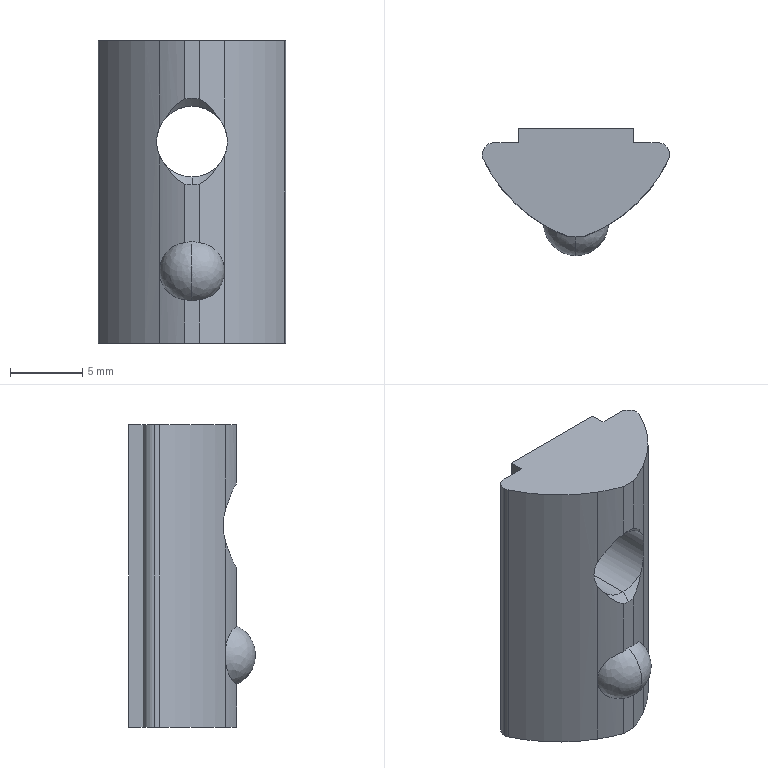Part | SolidWorks | features BaseBody 1 | 1 solid | 30 faces | box 13.001 x 8.797 x 21 mm | volume 1304 mm3 | cylinder 13 | plane 10 | cone 5 | spline 2 | commonest cylinder face diameters 20.854 x8 1.6 x3 4.917 x2
STEP:
#1=CARTESIAN_POINT('',(-0.0005,-8.797,-16.));
#2=VERTEX_POINT('',#1);
#3=CARTESIAN_POINT('',(-0.0005,-7.5,-18.038));
#4=VERTEX_POINT('',#3);
#5=CARTESIAN_POINT('',(-0.0005,-6.547,-16.));
#6=DIRECTION('',(1.,0.,0.));
#7=DIRECTION('',(0.,-1.,0.));
#8=AXIS2_PLACEMENT_3D('',#5,#6,#7);
#9=CIRCLE('',#8,2.25);
#10=EDGE_CURVE('',#2,#4,#9,.T.);
#11=ORIENTED_EDGE('',*,*,#10,.F.);
#12=CARTESIAN_POINT('',(-0.0005,-7.5,-13.962));
#13=VERTEX_POINT('',#12);
#14=CARTESIAN_POINT('',(-0.0005,-6.547,-16.));
#15=DIRECTION('',(-1.,0.,0.));
#16=DIRECTION('',(0.,-1.,0.));
#17=AXIS2_PLACEMENT_3D('',#14,#15,#16);
#18=CIRCLE('',#17,2.25);
#19=EDGE_CURVE('',#2,#13,#18,.T.);
#20=ORIENTED_EDGE('',*,*,#19,.T.);
#21=CARTESIAN_POINT('',(-0.5,-7.5,-14.024));
#22=VERTEX_POINT('',#21);
#23=CARTESIAN_POINT('',(-0.0005,-7.5,-16.));
#24=DIRECTION('',(0.,-1.,0.));
#25=DIRECTION('',(0.,0.,-1.));
#26=AXIS2_PLACEMENT_3D('',#23,#24,#25);
#27=CIRCLE('',#26,2.038);
#28=EDGE_CURVE('',#13,#22,#27,.T.);
#29=ORIENTED_EDGE('',*,*,#28,.T.);
#30=CARTESIAN_POINT('',(-2.246,-6.689,-16.));
#31=VERTEX_POINT('',#30);
#32=CARTESIAN_POINT('',(-0.5,-7.5,-14.024));
#33=CARTESIAN_POINT('',(-0.7396,-7.415,-14.043));
#34=CARTESIAN_POINT('',(-0.9674,-7.323,-14.106));
#35=CARTESIAN_POINT('',(-1.286,-7.184,-14.262));
#36=CARTESIAN_POINT('',(-1.386,-7.138,-14.324));
#37=CARTESIAN_POINT('',(-1.573,-7.049,-14.466));
#38=CARTESIAN_POINT('',(-1.662,-7.005,-14.548));
#39=CARTESIAN_POINT('',(-1.821,-6.924,-14.727));
#40=CARTESIAN_POINT('',(-1.892,-6.886,-14.824));
#41=CARTESIAN_POINT('',(-2.017,-6.819,-15.032));
#42=CARTESIAN_POINT('',(-2.071,-6.789,-15.144));
#43=CARTESIAN_POINT('',(-2.158,-6.74,-15.377));
#44=CARTESIAN_POINT('',(-2.19,-6.721,-15.497));
#45=CARTESIAN_POINT('',(-2.235,-6.696,-15.744));
#46=CARTESIAN_POINT('',(-2.246,-6.689,-15.872));
#47=CARTESIAN_POINT('',(-2.246,-6.689,-16.));
#48=B_SPLINE_CURVE_WITH_KNOTS('',3,(#32,#33,#34,#35,#36,#37,#38,#39,#40,#41,#42,#43,#44,#45,#46,#47),.UNSPECIFIED.,.F.,.F.,(4,2,2,2,2,2,2,4),(0.,0.0007548,0.001132,0.00151,0.001887,0.002264,0.002642,0.003019),.UNSPECIFIED.);
#49=EDGE_CURVE('',#22,#31,#48,.T.);
#50=ORIENTED_EDGE('',*,*,#49,.T.);
#51=CARTESIAN_POINT('',(-0.5,-7.5,-17.976));
#52=VERTEX_POINT('',#51);
#53=CARTESIAN_POINT('',(-0.5,-7.5,-17.976));
#54=CARTESIAN_POINT('',(-0.7396,-7.415,-17.957));
#55=CARTESIAN_POINT('',(-0.9674,-7.323,-17.894));
#56=CARTESIAN_POINT('',(-1.286,-7.184,-17.738));
#57=CARTESIAN_POINT('',(-1.386,-7.138,-17.676));
#58=CARTESIAN_POINT('',(-1.573,-7.049,-17.534));
#59=CARTESIAN_POINT('',(-1.662,-7.005,-17.452));
#60=CARTESIAN_POINT('',(-1.821,-6.924,-17.273));
#61=CARTESIAN_POINT('',(-1.892,-6.886,-17.176));
#62=CARTESIAN_POINT('',(-2.017,-6.819,-16.968));
#63=CARTESIAN_POINT('',(-2.071,-6.789,-16.856));
#64=CARTESIAN_POINT('',(-2.158,-6.74,-16.623));
#65=CARTESIAN_POINT('',(-2.19,-6.721,-16.503));
#66=CARTESIAN_POINT('',(-2.235,-6.696,-16.256));
#67=CARTESIAN_POINT('',(-2.246,-6.689,-16.128));
#68=CARTESIAN_POINT('',(-2.246,-6.689,-16.));
#69=B_SPLINE_CURVE_WITH_KNOTS('',3,(#53,#54,#55,#56,#57,#58,#59,#60,#61,#62,#63,#64,#65,#66,#67,#68),.UNSPECIFIED.,.F.,.F.,(4,2,2,2,2,2,2,4),(0.,0.0007548,0.001132,0.00151,0.001887,0.002264,0.002642,0.003019),.UNSPECIFIED.);
#70=EDGE_CURVE('',#52,#31,#69,.T.);
#71=ORIENTED_EDGE('',*,*,#70,.F.);
#72=CARTESIAN_POINT('',(-0.0005,-7.5,-16.));
#73=DIRECTION('',(0.,1.,0.));
#74=DIRECTION('',(0.,0.,-1.));
#75=AXIS2_PLACEMENT_3D('',#72,#73,#74);
#76=CIRCLE('',#75,2.038);
#77=EDGE_CURVE('',#4,#52,#76,.T.);
#78=ORIENTED_EDGE('',*,*,#77,.F.);
#79=EDGE_LOOP('',(#11,#20,#29,#50,#71,#78));
#80=FACE_OUTER_BOUND('',#79,.T.);
#81=CARTESIAN_POINT('',(-0.0005,-8.797,-16.));
#82=CARTESIAN_POINT('',(-0.0005,-8.797,-16.));
#83=CARTESIAN_POINT('',(-0.0005,-8.797,-16.));
#84=CARTESIAN_POINT('',(-0.0005,-8.797,-16.));
#85=CARTESIAN_POINT('',(-0.0005,-8.797,-14.738));
#86=CARTESIAN_POINT('',(-2.525,-8.797,-14.738));
#87=CARTESIAN_POINT('',(-2.525,-8.797,-17.262));
#88=CARTESIAN_POINT('',(-0.0005,-8.797,-17.262));
#89=CARTESIAN_POINT('',(-0.0005,-7.929,-13.822));
#90=CARTESIAN_POINT('',(-4.357,-7.929,-13.822));
#91=CARTESIAN_POINT('',(-4.357,-7.929,-18.178));
#92=CARTESIAN_POINT('',(-0.0005,-7.929,-18.178));
#93=CARTESIAN_POINT('',(-0.0005,-6.669,-13.753));
#94=CARTESIAN_POINT('',(-4.494,-6.669,-13.753));
#95=CARTESIAN_POINT('',(-4.494,-6.669,-18.247));
#96=CARTESIAN_POINT('',(-0.0005,-6.669,-18.247));
#97=(BOUNDED_SURFACE()B_SPLINE_SURFACE(3,3,((#81,#82,#83,#84),(#85,#86,#87,#88),(#89,#90,#91,#92),(#93,#94,#95,#96)),.UNSPECIFIED.,.F.,.F.,.T.)B_SPLINE_SURFACE_WITH_KNOTS((4,4),(4,4),(0.,1.),(0.,1.),.UNSPECIFIED.)GEOMETRIC_REPRESENTATION_ITEM()RATIONAL_B_SPLINE_SURFACE(((1.,0.3333,0.3333,1.),(0.8173,0.2724,0.2724,0.8173),(0.8173,0.2724,0.2724,0.8173),(1.,0.3333,0.3333,1.)))REPRESENTATION_ITEM('')SURFACE());
#98=ADVANCED_FACE('',(#80),#97,.T.);
#99=CARTESIAN_POINT('',(0.,-0.5415,-9.458));
#100=VERTEX_POINT('',#99);
#101=CARTESIAN_POINT('',(0.,-0.5415,-4.542));
#102=VERTEX_POINT('',#101);
#103=CARTESIAN_POINT('',(0.,-0.5415,-7.));
#104=DIRECTION('',(0.,1.,0.));
#105=DIRECTION('',(0.,0.,1.));
#106=AXIS2_PLACEMENT_3D('',#103,#104,#105);
#107=CIRCLE('',#106,2.458);
#108=EDGE_CURVE('',#100,#102,#107,.T.);
#109=ORIENTED_EDGE('',*,*,#108,.F.);
#110=CARTESIAN_POINT('',(0.,0.,-10.));
#111=VERTEX_POINT('',#110);
#112=CARTESIAN_POINT('',(0.,0.,-10.));
#113=DIRECTION('',(0.,0.7071,-0.7071));
#114=VECTOR('',#113,1000.);
#115=LINE('',#112,#114);
#116=EDGE_CURVE('',#100,#111,#115,.T.);
#117=ORIENTED_EDGE('',*,*,#116,.T.);
#118=CARTESIAN_POINT('',(0.,0.,-4.));
#119=VERTEX_POINT('',#118);
#120=CARTESIAN_POINT('',(0.,0.,-7.));
#121=DIRECTION('',(0.,-1.,0.));
#122=DIRECTION('',(0.,0.,1.));
#123=AXIS2_PLACEMENT_3D('',#120,#121,#122);
#124=CIRCLE('',#123,3.);
#125=EDGE_CURVE('',#119,#111,#124,.T.);
#126=ORIENTED_EDGE('',*,*,#125,.F.);
#127=CARTESIAN_POINT('',(0.,0.,-4.));
#128=DIRECTION('',(0.,0.7071,0.7071));
#129=VECTOR('',#128,1000.);
#130=LINE('',#127,#129);
#131=EDGE_CURVE('',#102,#119,#130,.T.);
#132=ORIENTED_EDGE('',*,*,#131,.F.);
#133=EDGE_LOOP('',(#109,#117,#126,#132));
#134=FACE_OUTER_BOUND('',#133,.T.);
#135=CARTESIAN_POINT('',(0.,0.,-7.));
#136=DIRECTION('',(0.,1.,0.));
#137=DIRECTION('',(0.,0.,1.));
#138=AXIS2_PLACEMENT_3D('',#135,#136,#137);
#139=CONICAL_SURFACE('',#138,3.,0.7854);
#140=ADVANCED_FACE('',(#134),#139,.F.);
#141=CARTESIAN_POINT('',(0.,-6.958,-9.458));
#142=VERTEX_POINT('',#141);
#143=CARTESIAN_POINT('',(-1.753,-6.959,-8.724));
#144=VERTEX_POINT('',#143);
#145=CARTESIAN_POINT('',(0.,-6.958,-7.));
#146=DIRECTION('',(0.,1.,0.));
#147=DIRECTION('',(0.,0.,1.));
#148=AXIS2_PLACEMENT_3D('',#145,#146,#147);
#149=CIRCLE('',#148,2.458);
#150=EDGE_CURVE('',#142,#144,#149,.T.);
#151=ORIENTED_EDGE('',*,*,#150,.F.);
#152=CARTESIAN_POINT('',(0.,-7.5,-9.458));
#153=DIRECTION('',(0.,1.,0.));
#154=VECTOR('',#153,1000.);
#155=LINE('',#152,#154);
#156=EDGE_CURVE('',#142,#100,#155,.T.);
#157=ORIENTED_EDGE('',*,*,#156,.T.);
#158=ORIENTED_EDGE('',*,*,#108,.T.);
#159=CARTESIAN_POINT('',(0.,-6.958,-4.542));
#160=VERTEX_POINT('',#159);
#161=CARTESIAN_POINT('',(0.,-7.5,-4.542));
#162=DIRECTION('',(0.,1.,0.));
#163=VECTOR('',#162,1000.);
#164=LINE('',#161,#163);
#165=EDGE_CURVE('',#160,#102,#164,.T.);
#166=ORIENTED_EDGE('',*,*,#165,.F.);
#167=CARTESIAN_POINT('',(-1.753,-6.959,-5.276));
#168=VERTEX_POINT('',#167);
#169=CARTESIAN_POINT('',(0.,-6.958,-7.));
#170=DIRECTION('',(0.,1.,0.));
#171=DIRECTION('',(0.,0.,1.));
#172=AXIS2_PLACEMENT_3D('',#169,#170,#171);
#173=CIRCLE('',#172,2.458);
#174=EDGE_CURVE('',#168,#160,#173,.T.);
#175=ORIENTED_EDGE('',*,*,#174,.F.);
#176=CARTESIAN_POINT('',(-2.246,-6.689,-6.));
#177=VERTEX_POINT('',#176);
#178=CARTESIAN_POINT('',(-2.246,-6.689,-6.));
#179=CARTESIAN_POINT('',(-2.123,-6.761,-5.724));
#180=CARTESIAN_POINT('',(-1.958,-6.854,-5.485));
#181=CARTESIAN_POINT('',(-1.753,-6.959,-5.276));
#182=B_SPLINE_CURVE_WITH_KNOTS('',3,(#178,#179,#180,#181),.UNSPECIFIED.,.F.,.F.,(4,4),(0.,0.0009162),.UNSPECIFIED.);
#183=EDGE_CURVE('',#177,#168,#182,.T.);
#184=ORIENTED_EDGE('',*,*,#183,.F.);
#185=CARTESIAN_POINT('',(-2.246,-6.689,-8.));
#186=VERTEX_POINT('',#185);
#187=CARTESIAN_POINT('',(-2.246,-6.689,-8.));
#188=CARTESIAN_POINT('',(-2.315,-6.649,-7.845));
#189=CARTESIAN_POINT('',(-2.368,-6.617,-7.683));
#190=CARTESIAN_POINT('',(-2.44,-6.573,-7.348));
#191=CARTESIAN_POINT('',(-2.458,-6.562,-7.173));
#192=CARTESIAN_POINT('',(-2.459,-6.562,-6.828));
#193=CARTESIAN_POINT('',(-2.44,-6.573,-6.655));
#194=CARTESIAN_POINT('',(-2.368,-6.617,-6.317));
#195=CARTESIAN_POINT('',(-2.315,-6.649,-6.155));
#196=CARTESIAN_POINT('',(-2.246,-6.689,-6.));
#197=B_SPLINE_CURVE_WITH_KNOTS('',3,(#187,#188,#189,#190,#191,#192,#193,#194,#195,#196),.UNSPECIFIED.,.F.,.F.,(4,2,2,2,4),(0.,0.0005173,0.001035,0.001552,0.002069),.UNSPECIFIED.);
#198=EDGE_CURVE('',#186,#177,#197,.T.);
#199=ORIENTED_EDGE('',*,*,#198,.F.);
#200=CARTESIAN_POINT('',(-1.753,-6.959,-8.724));
#201=CARTESIAN_POINT('',(-1.958,-6.854,-8.515));
#202=CARTESIAN_POINT('',(-2.123,-6.761,-8.276));
#203=CARTESIAN_POINT('',(-2.246,-6.689,-8.));
#204=B_SPLINE_CURVE_WITH_KNOTS('',3,(#200,#201,#202,#203),.UNSPECIFIED.,.F.,.F.,(4,4),(0.,0.0009162),.UNSPECIFIED.);
#205=EDGE_CURVE('',#144,#186,#204,.T.);
#206=ORIENTED_EDGE('',*,*,#205,.F.);
#207=EDGE_LOOP('',(#151,#157,#158,#166,#175,#184,#199,#206));
#208=FACE_OUTER_BOUND('',#207,.T.);
#209=CARTESIAN_POINT('',(0.,-7.5,-7.));
#210=DIRECTION('',(0.,1.,0.));
#211=DIRECTION('',(0.,0.,1.));
#212=AXIS2_PLACEMENT_3D('',#209,#210,#211);
#213=CYLINDRICAL_SURFACE('',#212,2.458);
#214=ADVANCED_FACE('',(#208),#213,.F.);
#215=CARTESIAN_POINT('',(-6.423,-2.143,0.));
#216=VERTEX_POINT('',#215);
#217=CARTESIAN_POINT('',(-6.5,-1.8,0.));
#218=VERTEX_POINT('',#217);
#219=CARTESIAN_POINT('',(-5.7,-1.8,0.));
#220=DIRECTION('',(0.,0.,-1.));
#221=DIRECTION('',(-1.,0.,0.));
#222=AXIS2_PLACEMENT_3D('',#219,#220,#221);
#223=CIRCLE('',#222,0.8);
#224=EDGE_CURVE('',#216,#218,#223,.T.);
#225=ORIENTED_EDGE('',*,*,#224,.T.);
#226=CARTESIAN_POINT('',(-6.5,-1.8,-21.));
#227=VERTEX_POINT('',#226);
#228=CARTESIAN_POINT('',(-6.5,-1.8,-21.));
#229=DIRECTION('',(0.,0.,-1.));
#230=VECTOR('',#229,1000.);
#231=LINE('',#228,#230);
#232=EDGE_CURVE('',#218,#227,#231,.T.);
#233=ORIENTED_EDGE('',*,*,#232,.T.);
#234=CARTESIAN_POINT('',(-6.423,-2.143,-21.));
#235=VERTEX_POINT('',#234);
#236=CARTESIAN_POINT('',(-5.7,-1.8,-21.));
#237=DIRECTION('',(0.,0.,1.));
#238=DIRECTION('',(-1.,0.,0.));
#239=AXIS2_PLACEMENT_3D('',#236,#237,#238);
#240=CIRCLE('',#239,0.8);
#241=EDGE_CURVE('',#227,#235,#240,.T.);
#242=ORIENTED_EDGE('',*,*,#241,.T.);
#243=CARTESIAN_POINT('',(-6.423,-2.143,-21.));
#244=DIRECTION('',(0.,0.,-1.));
#245=VECTOR('',#244,1000.);
#246=LINE('',#243,#245);
#247=EDGE_CURVE('',#216,#235,#246,.T.);
#248=ORIENTED_EDGE('',*,*,#247,.F.);
#249=EDGE_LOOP('',(#225,#233,#242,#248));
#250=FACE_OUTER_BOUND('',#249,.T.);
#251=CARTESIAN_POINT('',(-5.7,-1.8,-21.));
#252=DIRECTION('',(0.,0.,-1.));
#253=DIRECTION('',(-1.,0.,0.));
#254=AXIS2_PLACEMENT_3D('',#251,#252,#253);
#255=CYLINDRICAL_SURFACE('',#254,0.8);
#256=ADVANCED_FACE('',(#250),#255,.T.);
#257=CARTESIAN_POINT('',(1.752,-6.959,-8.724));
#258=VERTEX_POINT('',#257);
#259=CARTESIAN_POINT('',(0.,-6.958,-7.));
#260=DIRECTION('',(0.,1.,0.));
#261=DIRECTION('',(0.,0.,1.));
#262=AXIS2_PLACEMENT_3D('',#259,#260,#261);
#263=CIRCLE('',#262,2.458);
#264=EDGE_CURVE('',#258,#142,#263,.T.);
#265=ORIENTED_EDGE('',*,*,#264,.T.);
#266=CARTESIAN_POINT('',(0.,-7.5,-10.));
#267=VERTEX_POINT('',#266);
#268=CARTESIAN_POINT('',(0.,-7.5,-10.));
#269=DIRECTION('',(0.,-0.7071,-0.7071));
#270=VECTOR('',#269,1000.);
#271=LINE('',#268,#270);
#272=EDGE_CURVE('',#142,#267,#271,.T.);
#273=ORIENTED_EDGE('',*,*,#272,.T.);
#274=CARTESIAN_POINT('',(0.5,-7.5,-9.958));
#275=VERTEX_POINT('',#274);
#276=CARTESIAN_POINT('',(0.,-7.5,-7.));
#277=DIRECTION('',(0.,1.,0.));
#278=DIRECTION('',(0.,0.,-1.));
#279=AXIS2_PLACEMENT_3D('',#276,#277,#278);
#280=CIRCLE('',#279,3.);
#281=EDGE_CURVE('',#275,#267,#280,.T.);
#282=ORIENTED_EDGE('',*,*,#281,.F.);
#283=CARTESIAN_POINT('',(1.752,-6.959,-8.724));
#284=CARTESIAN_POINT('',(1.602,-7.036,-8.987));
#285=CARTESIAN_POINT('',(1.422,-7.123,-9.222));
#286=CARTESIAN_POINT('',(1.108,-7.262,-9.534));
#287=CARTESIAN_POINT('',(0.9946,-7.31,-9.632));
#288=CARTESIAN_POINT('',(0.7567,-7.405,-9.809));
#289=CARTESIAN_POINT('',(0.6317,-7.453,-9.888));
#290=CARTESIAN_POINT('',(0.5,-7.5,-9.958));
#291=B_SPLINE_CURVE_WITH_KNOTS('',3,(#283,#284,#285,#286,#287,#288,#289,#290),.UNSPECIFIED.,.F.,.F.,(4,2,2,4),(0.,0.0009244,0.001387,0.001849),.UNSPECIFIED.);
#292=EDGE_CURVE('',#258,#275,#291,.T.);
#293=ORIENTED_EDGE('',*,*,#292,.F.);
#294=EDGE_LOOP('',(#265,#273,#282,#293));
#295=FACE_OUTER_BOUND('',#294,.T.);
#296=CARTESIAN_POINT('',(0.,-7.5,-7.));
#297=DIRECTION('',(0.,-1.,0.));
#298=DIRECTION('',(0.,0.,-1.));
#299=AXIS2_PLACEMENT_3D('',#296,#297,#298);
#300=CONICAL_SURFACE('',#299,3.,0.7854);
#301=ADVANCED_FACE('',(#295),#300,.F.);
#302=CARTESIAN_POINT('',(4.,0.,-21.));
#303=VERTEX_POINT('',#302);
#304=CARTESIAN_POINT('',(-4.,0.,-21.));
#305=VERTEX_POINT('',#304);
#306=CARTESIAN_POINT('',(4.,0.,-21.));
#307=DIRECTION('',(-1.,0.,0.));
#308=VECTOR('',#307,1000.);
#309=LINE('',#306,#308);
#310=EDGE_CURVE('',#303,#305,#309,.T.);
#311=ORIENTED_EDGE('',*,*,#310,.T.);
#312=CARTESIAN_POINT('',(-4.,0.,0.));
#313=VERTEX_POINT('',#312);
#314=CARTESIAN_POINT('',(-4.,0.,-21.));
#315=DIRECTION('',(0.,0.,1.));
#316=VECTOR('',#315,1000.);
#317=LINE('',#314,#316);
#318=EDGE_CURVE('',#305,#313,#317,.T.);
#319=ORIENTED_EDGE('',*,*,#318,.T.);
#320=CARTESIAN_POINT('',(4.,0.,0.));
#321=VERTEX_POINT('',#320);
#322=CARTESIAN_POINT('',(4.,0.,0.));
#323=DIRECTION('',(1.,0.,0.));
#324=VECTOR('',#323,1000.);
#325=LINE('',#322,#324);
#326=EDGE_CURVE('',#313,#321,#325,.T.);
#327=ORIENTED_EDGE('',*,*,#326,.T.);
#328=CARTESIAN_POINT('',(4.,0.,-21.));
#329=DIRECTION('',(0.,0.,-1.));
#330=VECTOR('',#329,1000.);
#331=LINE('',#328,#330);
#332=EDGE_CURVE('',#321,#303,#331,.T.);
#333=ORIENTED_EDGE('',*,*,#332,.T.);
#334=EDGE_LOOP('',(#311,#319,#327,#333));
#335=FACE_OUTER_BOUND('',#334,.T.);
#336=ORIENTED_EDGE('',*,*,#125,.T.);
#337=CARTESIAN_POINT('',(0.,0.,-7.));
#338=DIRECTION('',(0.,-1.,0.));
#339=DIRECTION('',(0.,0.,1.));
#340=AXIS2_PLACEMENT_3D('',#337,#338,#339);
#341=CIRCLE('',#340,3.);
#342=EDGE_CURVE('',#111,#119,#341,.T.);
#343=ORIENTED_EDGE('',*,*,#342,.T.);
#344=EDGE_LOOP('',(#336,#343));
#345=FACE_BOUND('',#344,.T.);
#346=CARTESIAN_POINT('',(4.,0.,-21.));
#347=DIRECTION('',(0.,1.,0.));
#348=DIRECTION('',(0.,0.,1.));
#349=AXIS2_PLACEMENT_3D('',#346,#347,#348);
#350=PLANE('',#349);
#351=ADVANCED_FACE('',(#335,#345),#350,.T.);
#352=CARTESIAN_POINT('',(-4.,-1.,-21.));
#353=VERTEX_POINT('',#352);
#354=CARTESIAN_POINT('',(-4.,0.,-21.));
#355=DIRECTION('',(0.,-1.,0.));
#356=VECTOR('',#355,1000.);
#357=LINE('',#354,#356);
#358=EDGE_CURVE('',#305,#353,#357,.T.);
#359=ORIENTED_EDGE('',*,*,#358,.T.);
#360=CARTESIAN_POINT('',(-4.,-1.,0.));
#361=VERTEX_POINT('',#360);
#362=CARTESIAN_POINT('',(-4.,-1.,-21.));
#363=DIRECTION('',(0.,0.,1.));
#364=VECTOR('',#363,1000.);
#365=LINE('',#362,#364);
#366=EDGE_CURVE('',#353,#361,#365,.T.);
#367=ORIENTED_EDGE('',*,*,#366,.T.);
#368=CARTESIAN_POINT('',(-4.,0.,0.));
#369=DIRECTION('',(0.,1.,0.));
#370=VECTOR('',#369,1000.);
#371=LINE('',#368,#370);
#372=EDGE_CURVE('',#361,#313,#371,.T.);
#373=ORIENTED_EDGE('',*,*,#372,.T.);
#374=ORIENTED_EDGE('',*,*,#318,.F.);
#375=EDGE_LOOP('',(#359,#367,#373,#374));
#376=FACE_OUTER_BOUND('',#375,.T.);
#377=CARTESIAN_POINT('',(-4.,0.,-21.));
#378=DIRECTION('',(-1.,0.,0.));
#379=DIRECTION('',(0.,0.,1.));
#380=AXIS2_PLACEMENT_3D('',#377,#378,#379);
#381=PLANE('',#380);
#382=ADVANCED_FACE('',(#376),#381,.T.);
#383=ORIENTED_EDGE('',*,*,#358,.F.);
#384=ORIENTED_EDGE('',*,*,#310,.F.);
#385=CARTESIAN_POINT('',(4.,-1.,-21.));
#386=VERTEX_POINT('',#385);
#387=CARTESIAN_POINT('',(4.,-1.8,-21.));
#388=DIRECTION('',(0.,1.,0.));
#389=VECTOR('',#388,1000.);
#390=LINE('',#387,#389);
#391=EDGE_CURVE('',#386,#303,#390,.T.);
#392=ORIENTED_EDGE('',*,*,#391,.F.);
#393=CARTESIAN_POINT('',(5.7,-1.,-21.));
#394=VERTEX_POINT('',#393);
#395=CARTESIAN_POINT('',(5.7,-1.,-21.));
#396=DIRECTION('',(-1.,0.,0.));
#397=VECTOR('',#396,1000.);
#398=LINE('',#395,#397);
#399=EDGE_CURVE('',#394,#386,#398,.T.);
#400=ORIENTED_EDGE('',*,*,#399,.F.);
#401=CARTESIAN_POINT('',(6.423,-2.143,-21.));
#402=VERTEX_POINT('',#401);
#403=CARTESIAN_POINT('',(5.7,-1.8,-21.));
#404=DIRECTION('',(0.,0.,1.));
#405=DIRECTION('',(-1.,0.,0.));
#406=AXIS2_PLACEMENT_3D('',#403,#404,#405);
#407=CIRCLE('',#406,0.8);
#408=EDGE_CURVE('',#402,#394,#407,.T.);
#409=ORIENTED_EDGE('',*,*,#408,.F.);
#410=CARTESIAN_POINT('',(2.245,-6.689,-21.));
#411=VERTEX_POINT('',#410);
#412=CARTESIAN_POINT('',(-2.999,2.323,-21.));
#413=DIRECTION('',(0.,0.,1.));
#414=DIRECTION('',(-1.,0.,0.));
#415=AXIS2_PLACEMENT_3D('',#412,#413,#414);
#416=CIRCLE('',#415,10.427);
#417=EDGE_CURVE('',#411,#402,#416,.T.);
#418=ORIENTED_EDGE('',*,*,#417,.F.);
#419=CARTESIAN_POINT('',(0.5,-7.5,-21.));
#420=VERTEX_POINT('',#419);
#421=CARTESIAN_POINT('',(-3.003,2.321,-21.));
#422=DIRECTION('',(0.,0.,1.));
#423=DIRECTION('',(-1.,0.,0.));
#424=AXIS2_PLACEMENT_3D('',#421,#422,#423);
#425=CIRCLE('',#424,10.427);
#426=EDGE_CURVE('',#420,#411,#425,.T.);
#427=ORIENTED_EDGE('',*,*,#426,.F.);
#428=CARTESIAN_POINT('',(-0.5,-7.5,-21.));
#429=VERTEX_POINT('',#428);
#430=CARTESIAN_POINT('',(-0.5,-7.5,-21.));
#431=DIRECTION('',(1.,0.,0.));
#432=VECTOR('',#431,1000.);
#433=LINE('',#430,#432);
#434=EDGE_CURVE('',#429,#420,#433,.T.);
#435=ORIENTED_EDGE('',*,*,#434,.F.);
#436=CARTESIAN_POINT('',(-2.246,-6.689,-21.));
#437=VERTEX_POINT('',#436);
#438=CARTESIAN_POINT('',(3.001,2.322,-21.));
#439=DIRECTION('',(0.,0.,1.));
#440=DIRECTION('',(-1.,0.,0.));
#441=AXIS2_PLACEMENT_3D('',#438,#439,#440);
#442=CIRCLE('',#441,10.427);
#443=EDGE_CURVE('',#437,#429,#442,.T.);
#444=ORIENTED_EDGE('',*,*,#443,.F.);
#445=CARTESIAN_POINT('',(2.999,2.323,-21.));
#446=DIRECTION('',(0.,0.,1.));
#447=DIRECTION('',(-1.,0.,0.));
#448=AXIS2_PLACEMENT_3D('',#445,#446,#447);
#449=CIRCLE('',#448,10.427);
#450=EDGE_CURVE('',#235,#437,#449,.T.);
#451=ORIENTED_EDGE('',*,*,#450,.F.);
#452=ORIENTED_EDGE('',*,*,#241,.F.);
#453=CARTESIAN_POINT('',(-5.7,-1.,-21.));
#454=VERTEX_POINT('',#453);
#455=CARTESIAN_POINT('',(-5.7,-1.8,-21.));
#456=DIRECTION('',(0.,0.,1.));
#457=DIRECTION('',(-1.,0.,0.));
#458=AXIS2_PLACEMENT_3D('',#455,#456,#457);
#459=CIRCLE('',#458,0.8);
#460=EDGE_CURVE('',#454,#227,#459,.T.);
#461=ORIENTED_EDGE('',*,*,#460,.F.);
#462=CARTESIAN_POINT('',(-5.7,-1.,-21.));
#463=DIRECTION('',(-1.,0.,0.));
#464=VECTOR('',#463,1000.);
#465=LINE('',#462,#464);
#466=EDGE_CURVE('',#353,#454,#465,.T.);
#467=ORIENTED_EDGE('',*,*,#466,.F.);
#468=EDGE_LOOP('',(#383,#384,#392,#400,#409,#418,#427,#435,#444,#451,#452,#461,#467));
#469=FACE_OUTER_BOUND('',#468,.T.);
#470=CARTESIAN_POINT('',(-5.7,-1.8,-21.));
#471=DIRECTION('',(0.,0.,1.));
#472=DIRECTION('',(1.,0.,0.));
#473=AXIS2_PLACEMENT_3D('',#470,#471,#472);
#474=PLANE('',#473);
#475=ADVANCED_FACE('',(#469),#474,.F.);
#476=ORIENTED_EDGE('',*,*,#391,.T.);
#477=ORIENTED_EDGE('',*,*,#332,.F.);
#478=CARTESIAN_POINT('',(4.,-1.,0.));
#479=VERTEX_POINT('',#478);
#480=CARTESIAN_POINT('',(4.,-1.,0.));
#481=DIRECTION('',(0.,-1.,0.));
#482=VECTOR('',#481,1000.);
#483=LINE('',#480,#482);
#484=EDGE_CURVE('',#321,#479,#483,.T.);
#485=ORIENTED_EDGE('',*,*,#484,.T.);
#486=CARTESIAN_POINT('',(4.,-1.,-21.));
#487=DIRECTION('',(0.,0.,-1.));
#488=VECTOR('',#487,1000.);
#489=LINE('',#486,#488);
#490=EDGE_CURVE('',#479,#386,#489,.T.);
#491=ORIENTED_EDGE('',*,*,#490,.T.);
#492=EDGE_LOOP('',(#476,#477,#485,#491));
#493=FACE_OUTER_BOUND('',#492,.T.);
#494=CARTESIAN_POINT('',(4.,-1.,-21.));
#495=DIRECTION('',(1.,0.,0.));
#496=DIRECTION('',(0.,0.,-1.));
#497=AXIS2_PLACEMENT_3D('',#494,#495,#496);
#498=PLANE('',#497);
#499=ADVANCED_FACE('',(#493),#498,.T.);
#500=ORIENTED_EDGE('',*,*,#326,.F.);
#501=ORIENTED_EDGE('',*,*,#372,.F.);
#502=CARTESIAN_POINT('',(-5.7,-1.,0.));
#503=VERTEX_POINT('',#502);
#504=CARTESIAN_POINT('',(-5.7,-1.,0.));
#505=DIRECTION('',(-1.,0.,0.));
#506=VECTOR('',#505,1000.);
#507=LINE('',#504,#506);
#508=EDGE_CURVE('',#361,#503,#507,.T.);
#509=ORIENTED_EDGE('',*,*,#508,.T.);
#510=CARTESIAN_POINT('',(-5.7,-1.8,0.));
#511=DIRECTION('',(0.,0.,-1.));
#512=DIRECTION('',(-1.,0.,0.));
#513=AXIS2_PLACEMENT_3D('',#510,#511,#512);
#514=CIRCLE('',#513,0.8);
#515=EDGE_CURVE('',#218,#503,#514,.T.);
#516=ORIENTED_EDGE('',*,*,#515,.F.);
#517=ORIENTED_EDGE('',*,*,#224,.F.);
#518=CARTESIAN_POINT('',(-2.246,-6.689,0.));
#519=VERTEX_POINT('',#518);
#520=CARTESIAN_POINT('',(2.999,2.323,0.));
#521=DIRECTION('',(0.,0.,1.));
#522=DIRECTION('',(-1.,0.,0.));
#523=AXIS2_PLACEMENT_3D('',#520,#521,#522);
#524=CIRCLE('',#523,10.427);
#525=EDGE_CURVE('',#216,#519,#524,.T.);
#526=ORIENTED_EDGE('',*,*,#525,.T.);
#527=CARTESIAN_POINT('',(-0.5,-7.5,0.));
#528=VERTEX_POINT('',#527);
#529=CARTESIAN_POINT('',(3.001,2.322,0.));
#530=DIRECTION('',(0.,0.,1.));
#531=DIRECTION('',(-1.,0.,0.));
#532=AXIS2_PLACEMENT_3D('',#529,#530,#531);
#533=CIRCLE('',#532,10.427);
#534=EDGE_CURVE('',#519,#528,#533,.T.);
#535=ORIENTED_EDGE('',*,*,#534,.T.);
#536=CARTESIAN_POINT('',(0.5,-7.5,0.));
#537=VERTEX_POINT('',#536);
#538=CARTESIAN_POINT('',(-0.5,-7.5,0.));
#539=DIRECTION('',(-1.,0.,0.));
#540=VECTOR('',#539,1000.);
#541=LINE('',#538,#540);
#542=EDGE_CURVE('',#537,#528,#541,.T.);
#543=ORIENTED_EDGE('',*,*,#542,.F.);
#544=CARTESIAN_POINT('',(2.245,-6.689,0.));
#545=VERTEX_POINT('',#544);
#546=CARTESIAN_POINT('',(-3.003,2.321,0.));
#547=DIRECTION('',(0.,0.,1.));
#548=DIRECTION('',(-1.,0.,0.));
#549=AXIS2_PLACEMENT_3D('',#546,#547,#548);
#550=CIRCLE('',#549,10.427);
#551=EDGE_CURVE('',#537,#545,#550,.T.);
#552=ORIENTED_EDGE('',*,*,#551,.T.);
#553=CARTESIAN_POINT('',(6.423,-2.143,0.));
#554=VERTEX_POINT('',#553);
#555=CARTESIAN_POINT('',(-2.999,2.323,0.));
#556=DIRECTION('',(0.,0.,1.));
#557=DIRECTION('',(-1.,0.,0.));
#558=AXIS2_PLACEMENT_3D('',#555,#556,#557);
#559=CIRCLE('',#558,10.427);
#560=EDGE_CURVE('',#545,#554,#559,.T.);
#561=ORIENTED_EDGE('',*,*,#560,.T.);
#562=CARTESIAN_POINT('',(5.7,-1.,0.));
#563=VERTEX_POINT('',#562);
#564=CARTESIAN_POINT('',(5.7,-1.8,0.));
#565=DIRECTION('',(0.,0.,-1.));
#566=DIRECTION('',(-1.,0.,0.));
#567=AXIS2_PLACEMENT_3D('',#564,#565,#566);
#568=CIRCLE('',#567,0.8);
#569=EDGE_CURVE('',#563,#554,#568,.T.);
#570=ORIENTED_EDGE('',*,*,#569,.F.);
#571=CARTESIAN_POINT('',(-5.7,-1.,0.));
#572=DIRECTION('',(-1.,0.,0.));
#573=VECTOR('',#572,1000.);
#574=LINE('',#571,#573);
#575=EDGE_CURVE('',#563,#479,#574,.T.);
#576=ORIENTED_EDGE('',*,*,#575,.T.);
#577=ORIENTED_EDGE('',*,*,#484,.F.);
#578=EDGE_LOOP('',(#500,#501,#509,#516,#517,#526,#535,#543,#552,#561,#570,#576,#577));
#579=FACE_OUTER_BOUND('',#578,.T.);
#580=CARTESIAN_POINT('',(-5.7,-1.8,0.));
#581=DIRECTION('',(0.,0.,1.));
#582=DIRECTION('',(1.,0.,0.));
#583=AXIS2_PLACEMENT_3D('',#580,#581,#582);
#584=PLANE('',#583);
#585=ADVANCED_FACE('',(#579),#584,.T.);
#586=ORIENTED_EDGE('',*,*,#116,.F.);
#587=CARTESIAN_POINT('',(0.,-0.5415,-7.));
#588=DIRECTION('',(0.,1.,0.));
#589=DIRECTION('',(0.,0.,1.));
#590=AXIS2_PLACEMENT_3D('',#587,#588,#589);
#591=CIRCLE('',#590,2.458);
#592=EDGE_CURVE('',#102,#100,#591,.T.);
#593=ORIENTED_EDGE('',*,*,#592,.F.);
#594=ORIENTED_EDGE('',*,*,#131,.T.);
#595=ORIENTED_EDGE('',*,*,#342,.F.);
#596=EDGE_LOOP('',(#586,#593,#594,#595));
#597=FACE_OUTER_BOUND('',#596,.T.);
#598=CARTESIAN_POINT('',(0.,0.,-7.));
#599=DIRECTION('',(0.,1.,0.));
#600=DIRECTION('',(0.,0.,1.));
#601=AXIS2_PLACEMENT_3D('',#598,#599,#600);
#602=CONICAL_SURFACE('',#601,3.,0.7854);
#603=ADVANCED_FACE('',(#597),#602,.F.);
#604=ORIENTED_EDGE('',*,*,#466,.T.);
#605=CARTESIAN_POINT('',(-5.7,-1.,-21.));
#606=DIRECTION('',(0.,0.,1.));
#607=VECTOR('',#606,1000.);
#608=LINE('',#605,#607);
#609=EDGE_CURVE('',#454,#503,#608,.T.);
#610=ORIENTED_EDGE('',*,*,#609,.T.);
#611=ORIENTED_EDGE('',*,*,#508,.F.);
#612=ORIENTED_EDGE('',*,*,#366,.F.);
#613=EDGE_LOOP('',(#604,#610,#611,#612));
#614=FACE_OUTER_BOUND('',#613,.T.);
#615=CARTESIAN_POINT('',(-4.,-1.,-21.));
#616=DIRECTION('',(0.,1.,0.));
#617=DIRECTION('',(0.,0.,1.));
#618=AXIS2_PLACEMENT_3D('',#615,#616,#617);
#619=PLANE('',#618);
#620=ADVANCED_FACE('',(#614),#619,.T.);
#621=CARTESIAN_POINT('',(6.423,-2.143,-21.));
#622=DIRECTION('',(0.,0.,1.));
#623=VECTOR('',#622,1000.);
#624=LINE('',#621,#623);
#625=EDGE_CURVE('',#402,#554,#624,.T.);
#626=ORIENTED_EDGE('',*,*,#625,.T.);
#627=ORIENTED_EDGE('',*,*,#560,.F.);
#628=CARTESIAN_POINT('',(2.245,-6.689,-5.998));
#629=VERTEX_POINT('',#628);
#630=CARTESIAN_POINT('',(2.245,-6.689,-21.));
#631=DIRECTION('',(0.,0.,-1.));
#632=VECTOR('',#631,1000.);
#633=LINE('',#630,#632);
#634=EDGE_CURVE('',#545,#629,#633,.T.);
#635=ORIENTED_EDGE('',*,*,#634,.T.);
#636=CARTESIAN_POINT('',(2.245,-6.689,-8.002));
#637=VERTEX_POINT('',#636);
#638=CARTESIAN_POINT('',(2.245,-6.689,-5.998));
#639=CARTESIAN_POINT('',(2.314,-6.649,-6.154));
#640=CARTESIAN_POINT('',(2.367,-6.617,-6.315));
#641=CARTESIAN_POINT('',(2.44,-6.573,-6.651));
#642=CARTESIAN_POINT('',(2.458,-6.561,-6.827));
#643=CARTESIAN_POINT('',(2.459,-6.561,-7.172));
#644=CARTESIAN_POINT('',(2.44,-6.573,-7.346));
#645=CARTESIAN_POINT('',(2.368,-6.617,-7.684));
#646=CARTESIAN_POINT('',(2.314,-6.649,-7.846));
#647=CARTESIAN_POINT('',(2.245,-6.689,-8.002));
#648=B_SPLINE_CURVE_WITH_KNOTS('',3,(#638,#639,#640,#641,#642,#643,#644,#645,#646,#647),.UNSPECIFIED.,.F.,.F.,(4,2,2,2,4),(0.,0.0005185,0.001037,0.001556,0.002074),.UNSPECIFIED.);
#649=EDGE_CURVE('',#629,#637,#648,.T.);
#650=ORIENTED_EDGE('',*,*,#649,.T.);
#651=CARTESIAN_POINT('',(2.245,-6.689,-16.));
#652=VERTEX_POINT('',#651);
#653=CARTESIAN_POINT('',(2.245,-6.689,-21.));
#654=DIRECTION('',(0.,0.,-1.));
#655=VECTOR('',#654,1000.);
#656=LINE('',#653,#655);
#657=EDGE_CURVE('',#637,#652,#656,.T.);
#658=ORIENTED_EDGE('',*,*,#657,.T.);
#659=CARTESIAN_POINT('',(2.245,-6.689,-21.));
#660=DIRECTION('',(0.,0.,-1.));
#661=VECTOR('',#660,1000.);
#662=LINE('',#659,#661);
#663=EDGE_CURVE('',#652,#411,#662,.T.);
#664=ORIENTED_EDGE('',*,*,#663,.T.);
#665=ORIENTED_EDGE('',*,*,#417,.T.);
#666=EDGE_LOOP('',(#626,#627,#635,#650,#658,#664,#665));
#667=FACE_OUTER_BOUND('',#666,.T.);
#668=CARTESIAN_POINT('',(-2.999,2.323,-21.));
#669=DIRECTION('',(0.,0.,-1.));
#670=DIRECTION('',(-1.,0.,0.));
#671=AXIS2_PLACEMENT_3D('',#668,#669,#670);
#672=CYLINDRICAL_SURFACE('',#671,10.427);
#673=ADVANCED_FACE('',(#667),#672,.T.);
#674=ORIENTED_EDGE('',*,*,#426,.T.);
#675=ORIENTED_EDGE('',*,*,#663,.F.);
#676=CARTESIAN_POINT('',(0.5,-7.5,-17.976));
#677=VERTEX_POINT('',#676);
#678=CARTESIAN_POINT('',(2.245,-6.689,-16.));
#679=CARTESIAN_POINT('',(2.245,-6.689,-16.128));
#680=CARTESIAN_POINT('',(2.234,-6.696,-16.253));
#681=CARTESIAN_POINT('',(2.19,-6.721,-16.499));
#682=CARTESIAN_POINT('',(2.157,-6.74,-16.622));
#683=CARTESIAN_POINT('',(2.071,-6.788,-16.854));
#684=CARTESIAN_POINT('',(2.018,-6.818,-16.965));
#685=CARTESIAN_POINT('',(1.893,-6.885,-17.174));
#686=CARTESIAN_POINT('',(1.821,-6.923,-17.272));
#687=CARTESIAN_POINT('',(1.583,-7.045,-17.54));
#688=CARTESIAN_POINT('',(1.391,-7.138,-17.685));
#689=CARTESIAN_POINT('',(0.971,-7.322,-17.892));
#690=CARTESIAN_POINT('',(0.7393,-7.415,-17.956));
#691=CARTESIAN_POINT('',(0.5,-7.5,-17.976));
#692=B_SPLINE_CURVE_WITH_KNOTS('',3,(#678,#679,#680,#681,#682,#683,#684,#685,#686,#687,#688,#689,#690,#691),.UNSPECIFIED.,.F.,.F.,(4,2,2,2,2,2,4),(0.,0.000377,0.0007541,0.001131,0.001508,0.002262,0.003016),.UNSPECIFIED.);
#693=EDGE_CURVE('',#652,#677,#692,.T.);
#694=ORIENTED_EDGE('',*,*,#693,.T.);
#695=CARTESIAN_POINT('',(0.5,-7.5,-21.));
#696=DIRECTION('',(0.,0.,-1.));
#697=VECTOR('',#696,1000.);
#698=LINE('',#695,#697);
#699=EDGE_CURVE('',#677,#420,#698,.T.);
#700=ORIENTED_EDGE('',*,*,#699,.T.);
#701=EDGE_LOOP('',(#674,#675,#694,#700));
#702=FACE_OUTER_BOUND('',#701,.T.);
#703=CARTESIAN_POINT('',(-3.003,2.321,-21.));
#704=DIRECTION('',(0.,0.,-1.));
#705=DIRECTION('',(-1.,0.,0.));
#706=AXIS2_PLACEMENT_3D('',#703,#704,#705);
#707=CYLINDRICAL_SURFACE('',#706,10.427);
#708=ADVANCED_FACE('',(#702),#707,.T.);
#709=ORIENTED_EDGE('',*,*,#443,.T.);
#710=CARTESIAN_POINT('',(-0.5,-7.5,-21.));
#711=DIRECTION('',(0.,0.,1.));
#712=VECTOR('',#711,1000.);
#713=LINE('',#710,#712);
#714=EDGE_CURVE('',#429,#52,#713,.T.);
#715=ORIENTED_EDGE('',*,*,#714,.T.);
#716=ORIENTED_EDGE('',*,*,#70,.T.);
#717=CARTESIAN_POINT('',(-2.246,-6.689,-21.));
#718=DIRECTION('',(0.,0.,-1.));
#719=VECTOR('',#718,1000.);
#720=LINE('',#717,#719);
#721=EDGE_CURVE('',#31,#437,#720,.T.);
#722=ORIENTED_EDGE('',*,*,#721,.T.);
#723=EDGE_LOOP('',(#709,#715,#716,#722));
#724=FACE_OUTER_BOUND('',#723,.T.);
#725=CARTESIAN_POINT('',(3.001,2.322,-21.));
#726=DIRECTION('',(0.,0.,-1.));
#727=DIRECTION('',(-1.,0.,0.));
#728=AXIS2_PLACEMENT_3D('',#725,#726,#727);
#729=CYLINDRICAL_SURFACE('',#728,10.427);
#730=ADVANCED_FACE('',(#724),#729,.T.);
#731=ORIENTED_EDGE('',*,*,#247,.T.);
#732=ORIENTED_EDGE('',*,*,#450,.T.);
#733=ORIENTED_EDGE('',*,*,#721,.F.);
#734=CARTESIAN_POINT('',(-2.246,-6.689,-21.));
#735=DIRECTION('',(0.,0.,1.));
#736=VECTOR('',#735,1000.);
#737=LINE('',#734,#736);
#738=EDGE_CURVE('',#31,#186,#737,.T.);
#739=ORIENTED_EDGE('',*,*,#738,.T.);
#740=ORIENTED_EDGE('',*,*,#198,.T.);
#741=CARTESIAN_POINT('',(-2.246,-6.689,-21.));
#742=DIRECTION('',(0.,0.,1.));
#743=VECTOR('',#742,1000.);
#744=LINE('',#741,#743);
#745=EDGE_CURVE('',#177,#519,#744,.T.);
#746=ORIENTED_EDGE('',*,*,#745,.T.);
#747=ORIENTED_EDGE('',*,*,#525,.F.);
#748=EDGE_LOOP('',(#731,#732,#733,#739,#740,#746,#747));
#749=FACE_OUTER_BOUND('',#748,.T.);
#750=CARTESIAN_POINT('',(2.999,2.323,-21.));
#751=DIRECTION('',(0.,0.,-1.));
#752=DIRECTION('',(-1.,0.,0.));
#753=AXIS2_PLACEMENT_3D('',#750,#751,#752);
#754=CYLINDRICAL_SURFACE('',#753,10.427);
#755=ADVANCED_FACE('',(#749),#754,.T.);
#756=ORIENTED_EDGE('',*,*,#399,.T.);
#757=ORIENTED_EDGE('',*,*,#490,.F.);
#758=ORIENTED_EDGE('',*,*,#575,.F.);
#759=CARTESIAN_POINT('',(5.7,-1.,-21.));
#760=DIRECTION('',(0.,0.,-1.));
#761=VECTOR('',#760,1000.);
#762=LINE('',#759,#761);
#763=EDGE_CURVE('',#563,#394,#762,.T.);
#764=ORIENTED_EDGE('',*,*,#763,.T.);
#765=EDGE_LOOP('',(#756,#757,#758,#764));
#766=FACE_OUTER_BOUND('',#765,.T.);
#767=CARTESIAN_POINT('',(5.7,-1.,-21.));
#768=DIRECTION('',(0.,1.,0.));
#769=DIRECTION('',(0.,0.,1.));
#770=AXIS2_PLACEMENT_3D('',#767,#768,#769);
#771=PLANE('',#770);
#772=ADVANCED_FACE('',(#766),#771,.T.);
#773=ORIENTED_EDGE('',*,*,#551,.F.);
#774=CARTESIAN_POINT('',(0.5,-7.5,-4.042));
#775=VERTEX_POINT('',#774);
#776=CARTESIAN_POINT('',(0.5,-7.5,-21.));
#777=DIRECTION('',(0.,0.,-1.));
#778=VECTOR('',#777,1000.);
#779=LINE('',#776,#778);
#780=EDGE_CURVE('',#537,#775,#779,.T.);
#781=ORIENTED_EDGE('',*,*,#780,.T.);
#782=CARTESIAN_POINT('',(1.752,-6.959,-5.276));
#783=VERTEX_POINT('',#782);
#784=CARTESIAN_POINT('',(0.5,-7.5,-4.042));
#785=CARTESIAN_POINT('',(0.7635,-7.406,-4.182));
#786=CARTESIAN_POINT('',(0.9981,-7.311,-4.358));
#787=CARTESIAN_POINT('',(1.314,-7.171,-4.67));
#788=CARTESIAN_POINT('',(1.413,-7.125,-4.782));
#789=CARTESIAN_POINT('',(1.594,-7.038,-5.019));
#790=CARTESIAN_POINT('',(1.677,-6.997,-5.144));
#791=CARTESIAN_POINT('',(1.752,-6.959,-5.276));
#792=B_SPLINE_CURVE_WITH_KNOTS('',3,(#784,#785,#786,#787,#788,#789,#790,#791),.UNSPECIFIED.,.F.,.F.,(4,2,2,4),(0.,0.0009248,0.001387,0.00185),.UNSPECIFIED.);
#793=EDGE_CURVE('',#775,#783,#792,.T.);
#794=ORIENTED_EDGE('',*,*,#793,.T.);
#795=CARTESIAN_POINT('',(1.752,-6.959,-5.276));
#796=CARTESIAN_POINT('',(1.957,-6.854,-5.483));
#797=CARTESIAN_POINT('',(2.122,-6.761,-5.722));
#798=CARTESIAN_POINT('',(2.245,-6.689,-5.998));
#799=B_SPLINE_CURVE_WITH_KNOTS('',3,(#795,#796,#797,#798),.UNSPECIFIED.,.F.,.F.,(4,4),(0.,0.000915),.UNSPECIFIED.);
#800=EDGE_CURVE('',#783,#629,#799,.T.);
#801=ORIENTED_EDGE('',*,*,#800,.T.);
#802=ORIENTED_EDGE('',*,*,#634,.F.);
#803=EDGE_LOOP('',(#773,#781,#794,#801,#802));
#804=FACE_OUTER_BOUND('',#803,.T.);
#805=CARTESIAN_POINT('',(-3.003,2.321,-21.));
#806=DIRECTION('',(0.,0.,-1.));
#807=DIRECTION('',(-1.,0.,0.));
#808=AXIS2_PLACEMENT_3D('',#805,#806,#807);
#809=CYLINDRICAL_SURFACE('',#808,10.427);
#810=ADVANCED_FACE('',(#804),#809,.T.);
#811=CARTESIAN_POINT('',(-0.5,-7.5,-4.042));
#812=VERTEX_POINT('',#811);
#813=CARTESIAN_POINT('',(-0.5,-7.5,-21.));
#814=DIRECTION('',(0.,0.,1.));
#815=VECTOR('',#814,1000.);
#816=LINE('',#813,#815);
#817=EDGE_CURVE('',#812,#528,#816,.T.);
#818=ORIENTED_EDGE('',*,*,#817,.T.);
#819=ORIENTED_EDGE('',*,*,#534,.F.);
#820=ORIENTED_EDGE('',*,*,#745,.F.);
#821=ORIENTED_EDGE('',*,*,#183,.T.);
#822=CARTESIAN_POINT('',(-1.753,-6.959,-5.276));
#823=CARTESIAN_POINT('',(-1.603,-7.036,-5.013));
#824=CARTESIAN_POINT('',(-1.423,-7.123,-4.778));
#825=CARTESIAN_POINT('',(-1.108,-7.262,-4.466));
#826=CARTESIAN_POINT('',(-0.9949,-7.31,-4.368));
#827=CARTESIAN_POINT('',(-0.7569,-7.405,-4.191));
#828=CARTESIAN_POINT('',(-0.6318,-7.453,-4.112));
#829=CARTESIAN_POINT('',(-0.5,-7.5,-4.042));
#830=B_SPLINE_CURVE_WITH_KNOTS('',3,(#822,#823,#824,#825,#826,#827,#828,#829),.UNSPECIFIED.,.F.,.F.,(4,2,2,4),(0.,0.000925,0.001387,0.00185),.UNSPECIFIED.);
#831=EDGE_CURVE('',#168,#812,#830,.T.);
#832=ORIENTED_EDGE('',*,*,#831,.T.);
#833=EDGE_LOOP('',(#818,#819,#820,#821,#832));
#834=FACE_OUTER_BOUND('',#833,.T.);
#835=CARTESIAN_POINT('',(3.001,2.322,-21.));
#836=DIRECTION('',(0.,0.,-1.));
#837=DIRECTION('',(-1.,0.,0.));
#838=AXIS2_PLACEMENT_3D('',#835,#836,#837);
#839=CYLINDRICAL_SURFACE('',#838,10.427);
#840=ADVANCED_FACE('',(#834),#839,.T.);
#841=ORIENTED_EDGE('',*,*,#156,.F.);
#842=ORIENTED_EDGE('',*,*,#264,.F.);
#843=CARTESIAN_POINT('',(2.245,-6.689,-8.002));
#844=CARTESIAN_POINT('',(2.122,-6.761,-8.278));
#845=CARTESIAN_POINT('',(1.957,-6.854,-8.517));
#846=CARTESIAN_POINT('',(1.752,-6.959,-8.724));
#847=B_SPLINE_CURVE_WITH_KNOTS('',3,(#843,#844,#845,#846),.UNSPECIFIED.,.F.,.F.,(4,4),(0.,0.000915),.UNSPECIFIED.);
#848=EDGE_CURVE('',#637,#258,#847,.T.);
#849=ORIENTED_EDGE('',*,*,#848,.F.);
#850=ORIENTED_EDGE('',*,*,#649,.F.);
#851=ORIENTED_EDGE('',*,*,#800,.F.);
#852=CARTESIAN_POINT('',(0.,-6.958,-7.));
#853=DIRECTION('',(0.,1.,0.));
#854=DIRECTION('',(0.,0.,1.));
#855=AXIS2_PLACEMENT_3D('',#852,#853,#854);
#856=CIRCLE('',#855,2.458);
#857=EDGE_CURVE('',#160,#783,#856,.T.);
#858=ORIENTED_EDGE('',*,*,#857,.F.);
#859=ORIENTED_EDGE('',*,*,#165,.T.);
#860=ORIENTED_EDGE('',*,*,#592,.T.);
#861=EDGE_LOOP('',(#841,#842,#849,#850,#851,#858,#859,#860));
#862=FACE_OUTER_BOUND('',#861,.T.);
#863=CARTESIAN_POINT('',(0.,-7.5,-7.));
#864=DIRECTION('',(0.,1.,0.));
#865=DIRECTION('',(0.,0.,1.));
#866=AXIS2_PLACEMENT_3D('',#863,#864,#865);
#867=CYLINDRICAL_SURFACE('',#866,2.458);
#868=ADVANCED_FACE('',(#862),#867,.F.);
#869=ORIENTED_EDGE('',*,*,#232,.F.);
#870=ORIENTED_EDGE('',*,*,#515,.T.);
#871=ORIENTED_EDGE('',*,*,#609,.F.);
#872=ORIENTED_EDGE('',*,*,#460,.T.);
#873=EDGE_LOOP('',(#869,#870,#871,#872));
#874=FACE_OUTER_BOUND('',#873,.T.);
#875=CARTESIAN_POINT('',(-5.7,-1.8,-21.));
#876=DIRECTION('',(0.,0.,-1.));
#877=DIRECTION('',(-1.,0.,0.));
#878=AXIS2_PLACEMENT_3D('',#875,#876,#877);
#879=CYLINDRICAL_SURFACE('',#878,0.8);
#880=ADVANCED_FACE('',(#874),#879,.T.);
#881=ORIENTED_EDGE('',*,*,#408,.T.);
#882=ORIENTED_EDGE('',*,*,#763,.F.);
#883=ORIENTED_EDGE('',*,*,#569,.T.);
#884=ORIENTED_EDGE('',*,*,#625,.F.);
#885=EDGE_LOOP('',(#881,#882,#883,#884));
#886=FACE_OUTER_BOUND('',#885,.T.);
#887=CARTESIAN_POINT('',(5.7,-1.8,-21.));
#888=DIRECTION('',(0.,0.,-1.));
#889=DIRECTION('',(-1.,0.,0.));
#890=AXIS2_PLACEMENT_3D('',#887,#888,#889);
#891=CYLINDRICAL_SURFACE('',#890,0.8);
#892=ADVANCED_FACE('',(#886),#891,.T.);
#893=ORIENTED_EDGE('',*,*,#292,.T.);
#894=CARTESIAN_POINT('',(0.5,-7.5,-14.024));
#895=VERTEX_POINT('',#894);
#896=CARTESIAN_POINT('',(0.5,-7.5,-21.));
#897=DIRECTION('',(0.,0.,-1.));
#898=VECTOR('',#897,1000.);
#899=LINE('',#896,#898);
#900=EDGE_CURVE('',#275,#895,#899,.T.);
#901=ORIENTED_EDGE('',*,*,#900,.T.);
#902=CARTESIAN_POINT('',(0.5,-7.5,-14.024));
#903=CARTESIAN_POINT('',(0.7395,-7.415,-14.044));
#904=CARTESIAN_POINT('',(0.9672,-7.323,-14.106));
#905=CARTESIAN_POINT('',(1.286,-7.184,-14.263));
#906=CARTESIAN_POINT('',(1.385,-7.138,-14.324));
#907=CARTESIAN_POINT('',(1.573,-7.049,-14.467));
#908=CARTESIAN_POINT('',(1.661,-7.005,-14.548));
#909=CARTESIAN_POINT('',(1.821,-6.924,-14.727));
#910=CARTESIAN_POINT('',(1.892,-6.886,-14.824));
#911=CARTESIAN_POINT('',(2.016,-6.819,-15.032));
#912=CARTESIAN_POINT('',(2.07,-6.789,-15.145));
#913=CARTESIAN_POINT('',(2.157,-6.74,-15.377));
#914=CARTESIAN_POINT('',(2.189,-6.721,-15.497));
#915=CARTESIAN_POINT('',(2.234,-6.696,-15.744));
#916=CARTESIAN_POINT('',(2.245,-6.689,-15.872));
#917=CARTESIAN_POINT('',(2.245,-6.689,-16.));
#918=B_SPLINE_CURVE_WITH_KNOTS('',3,(#902,#903,#904,#905,#906,#907,#908,#909,#910,#911,#912,#913,#914,#915,#916,#917),.UNSPECIFIED.,.F.,.F.,(4,2,2,2,2,2,2,4),(0.,0.0007545,0.001132,0.001509,0.001886,0.002264,0.002641,0.003018),.UNSPECIFIED.);
#919=EDGE_CURVE('',#895,#652,#918,.T.);
#920=ORIENTED_EDGE('',*,*,#919,.T.);
#921=ORIENTED_EDGE('',*,*,#657,.F.);
#922=ORIENTED_EDGE('',*,*,#848,.T.);
#923=EDGE_LOOP('',(#893,#901,#920,#921,#922));
#924=FACE_OUTER_BOUND('',#923,.T.);
#925=CARTESIAN_POINT('',(-3.003,2.321,-21.));
#926=DIRECTION('',(0.,0.,-1.));
#927=DIRECTION('',(-1.,0.,0.));
#928=AXIS2_PLACEMENT_3D('',#925,#926,#927);
#929=CYLINDRICAL_SURFACE('',#928,10.427);
#930=ADVANCED_FACE('',(#924),#929,.T.);
#931=ORIENTED_EDGE('',*,*,#434,.T.);
#932=ORIENTED_EDGE('',*,*,#699,.F.);
#933=CARTESIAN_POINT('',(-0.0005,-7.5,-16.));
#934=DIRECTION('',(0.,1.,0.));
#935=DIRECTION('',(0.,0.,-1.));
#936=AXIS2_PLACEMENT_3D('',#933,#934,#935);
#937=CIRCLE('',#936,2.038);
#938=EDGE_CURVE('',#677,#4,#937,.T.);
#939=ORIENTED_EDGE('',*,*,#938,.T.);
#940=ORIENTED_EDGE('',*,*,#77,.T.);
#941=ORIENTED_EDGE('',*,*,#714,.F.);
#942=EDGE_LOOP('',(#931,#932,#939,#940,#941));
#943=FACE_OUTER_BOUND('',#942,.T.);
#944=CARTESIAN_POINT('',(-0.5,-7.5,-21.));
#945=DIRECTION('',(0.,-1.,0.));
#946=DIRECTION('',(0.,0.,-1.));
#947=AXIS2_PLACEMENT_3D('',#944,#945,#946);
#948=PLANE('',#947);
#949=ADVANCED_FACE('',(#943),#948,.T.);
#950=ORIENTED_EDGE('',*,*,#19,.F.);
#951=ORIENTED_EDGE('',*,*,#10,.T.);
#952=ORIENTED_EDGE('',*,*,#938,.F.);
#953=ORIENTED_EDGE('',*,*,#693,.F.);
#954=ORIENTED_EDGE('',*,*,#919,.F.);
#955=CARTESIAN_POINT('',(-0.0005,-7.5,-16.));
#956=DIRECTION('',(0.,-1.,0.));
#957=DIRECTION('',(0.,0.,-1.));
#958=AXIS2_PLACEMENT_3D('',#955,#956,#957);
#959=CIRCLE('',#958,2.038);
#960=EDGE_CURVE('',#895,#13,#959,.T.);
#961=ORIENTED_EDGE('',*,*,#960,.T.);
#962=EDGE_LOOP('',(#950,#951,#952,#953,#954,#961));
#963=FACE_OUTER_BOUND('',#962,.T.);
#964=CARTESIAN_POINT('',(-0.0005,-8.797,-16.));
#965=CARTESIAN_POINT('',(-0.0005,-8.797,-16.));
#966=CARTESIAN_POINT('',(-0.0005,-8.797,-16.));
#967=CARTESIAN_POINT('',(-0.0005,-8.797,-16.));
#968=CARTESIAN_POINT('',(-0.0005,-8.797,-17.262));
#969=CARTESIAN_POINT('',(2.524,-8.797,-17.262));
#970=CARTESIAN_POINT('',(2.524,-8.797,-14.738));
#971=CARTESIAN_POINT('',(-0.0005,-8.797,-14.738));
#972=CARTESIAN_POINT('',(-0.0005,-7.929,-18.178));
#973=CARTESIAN_POINT('',(4.356,-7.929,-18.178));
#974=CARTESIAN_POINT('',(4.356,-7.929,-13.822));
#975=CARTESIAN_POINT('',(-0.0005,-7.929,-13.822));
#976=CARTESIAN_POINT('',(-0.0005,-6.669,-18.247));
#977=CARTESIAN_POINT('',(4.493,-6.669,-18.247));
#978=CARTESIAN_POINT('',(4.493,-6.669,-13.753));
#979=CARTESIAN_POINT('',(-0.0005,-6.669,-13.753));
#980=(BOUNDED_SURFACE()B_SPLINE_SURFACE(3,3,((#964,#965,#966,#967),(#968,#969,#970,#971),(#972,#973,#974,#975),(#976,#977,#978,#979)),.UNSPECIFIED.,.F.,.F.,.F.)B_SPLINE_SURFACE_WITH_KNOTS((4,4),(4,4),(0.,1.),(0.,1.),.UNSPECIFIED.)GEOMETRIC_REPRESENTATION_ITEM()RATIONAL_B_SPLINE_SURFACE(((1.,0.3333,0.3333,1.),(0.8173,0.2724,0.2724,0.8173),(0.8173,0.2724,0.2724,0.8173),(1.,0.3333,0.3333,1.)))REPRESENTATION_ITEM('')SURFACE());
#981=ADVANCED_FACE('',(#963),#980,.T.);
#982=ORIENTED_EDGE('',*,*,#205,.T.);
#983=ORIENTED_EDGE('',*,*,#738,.F.);
#984=ORIENTED_EDGE('',*,*,#49,.F.);
#985=CARTESIAN_POINT('',(-0.5,-7.5,-9.958));
#986=VERTEX_POINT('',#985);
#987=CARTESIAN_POINT('',(-0.5,-7.5,-21.));
#988=DIRECTION('',(0.,0.,1.));
#989=VECTOR('',#988,1000.);
#990=LINE('',#987,#989);
#991=EDGE_CURVE('',#22,#986,#990,.T.);
#992=ORIENTED_EDGE('',*,*,#991,.T.);
#993=CARTESIAN_POINT('',(-0.5,-7.5,-9.958));
#994=CARTESIAN_POINT('',(-0.7637,-7.406,-9.818));
#995=CARTESIAN_POINT('',(-0.9985,-7.311,-9.642));
#996=CARTESIAN_POINT('',(-1.314,-7.171,-9.33));
#997=CARTESIAN_POINT('',(-1.413,-7.125,-9.217));
#998=CARTESIAN_POINT('',(-1.595,-7.038,-8.98));
#999=CARTESIAN_POINT('',(-1.678,-6.997,-8.855));
#1000=CARTESIAN_POINT('',(-1.753,-6.959,-8.724));
#1001=B_SPLINE_CURVE_WITH_KNOTS('',3,(#993,#994,#995,#996,#997,#998,#999,#1000),.UNSPECIFIED.,.F.,.F.,(4,2,2,4),(0.,0.0009253,0.001388,0.001851),.UNSPECIFIED.);
#1002=EDGE_CURVE('',#986,#144,#1001,.T.);
#1003=ORIENTED_EDGE('',*,*,#1002,.T.);
#1004=EDGE_LOOP('',(#982,#983,#984,#992,#1003));
#1005=FACE_OUTER_BOUND('',#1004,.T.);
#1006=CARTESIAN_POINT('',(3.001,2.322,-21.));
#1007=DIRECTION('',(0.,0.,-1.));
#1008=DIRECTION('',(-1.,0.,0.));
#1009=AXIS2_PLACEMENT_3D('',#1006,#1007,#1008);
#1010=CYLINDRICAL_SURFACE('',#1009,10.427);
#1011=ADVANCED_FACE('',(#1005),#1010,.T.);
#1012=ORIENTED_EDGE('',*,*,#780,.F.);
#1013=ORIENTED_EDGE('',*,*,#542,.T.);
#1014=ORIENTED_EDGE('',*,*,#817,.F.);
#1015=CARTESIAN_POINT('',(0.,-7.5,-7.));
#1016=DIRECTION('',(0.,1.,0.));
#1017=DIRECTION('',(0.,0.,-1.));
#1018=AXIS2_PLACEMENT_3D('',#1015,#1016,#1017);
#1019=CIRCLE('',#1018,3.);
#1020=EDGE_CURVE('',#812,#775,#1019,.T.);
#1021=ORIENTED_EDGE('',*,*,#1020,.T.);
#1022=EDGE_LOOP('',(#1012,#1013,#1014,#1021));
#1023=FACE_OUTER_BOUND('',#1022,.T.);
#1024=CARTESIAN_POINT('',(-0.5,-7.5,-21.));
#1025=DIRECTION('',(0.,-1.,0.));
#1026=DIRECTION('',(0.,0.,-1.));
#1027=AXIS2_PLACEMENT_3D('',#1024,#1025,#1026);
#1028=PLANE('',#1027);
#1029=ADVANCED_FACE('',(#1023),#1028,.T.);
#1030=ORIENTED_EDGE('',*,*,#793,.F.);
#1031=ORIENTED_EDGE('',*,*,#1020,.F.);
#1032=ORIENTED_EDGE('',*,*,#831,.F.);
#1033=ORIENTED_EDGE('',*,*,#174,.T.);
#1034=ORIENTED_EDGE('',*,*,#857,.T.);
#1035=EDGE_LOOP('',(#1030,#1031,#1032,#1033,#1034));
#1036=FACE_OUTER_BOUND('',#1035,.T.);
#1037=CARTESIAN_POINT('',(0.,-7.5,-7.));
#1038=DIRECTION('',(0.,-1.,0.));
#1039=DIRECTION('',(0.,0.,-1.));
#1040=AXIS2_PLACEMENT_3D('',#1037,#1038,#1039);
#1041=CONICAL_SURFACE('',#1040,3.,0.7854);
#1042=ADVANCED_FACE('',(#1036),#1041,.F.);
#1043=ORIENTED_EDGE('',*,*,#272,.F.);
#1044=ORIENTED_EDGE('',*,*,#150,.T.);
#1045=ORIENTED_EDGE('',*,*,#1002,.F.);
#1046=CARTESIAN_POINT('',(0.,-7.5,-7.));
#1047=DIRECTION('',(0.,1.,0.));
#1048=DIRECTION('',(0.,0.,-1.));
#1049=AXIS2_PLACEMENT_3D('',#1046,#1047,#1048);
#1050=CIRCLE('',#1049,3.);
#1051=EDGE_CURVE('',#267,#986,#1050,.T.);
#1052=ORIENTED_EDGE('',*,*,#1051,.F.);
#1053=EDGE_LOOP('',(#1043,#1044,#1045,#1052));
#1054=FACE_OUTER_BOUND('',#1053,.T.);
#1055=CARTESIAN_POINT('',(0.,-7.5,-7.));
#1056=DIRECTION('',(0.,-1.,0.));
#1057=DIRECTION('',(0.,0.,-1.));
#1058=AXIS2_PLACEMENT_3D('',#1055,#1056,#1057);
#1059=CONICAL_SURFACE('',#1058,3.,0.7854);
#1060=ADVANCED_FACE('',(#1054),#1059,.F.);
#1061=ORIENTED_EDGE('',*,*,#281,.T.);
#1062=ORIENTED_EDGE('',*,*,#1051,.T.);
#1063=ORIENTED_EDGE('',*,*,#991,.F.);
#1064=ORIENTED_EDGE('',*,*,#28,.F.);
#1065=ORIENTED_EDGE('',*,*,#960,.F.);
#1066=ORIENTED_EDGE('',*,*,#900,.F.);
#1067=EDGE_LOOP('',(#1061,#1062,#1063,#1064,#1065,#1066));
#1068=FACE_OUTER_BOUND('',#1067,.T.);
#1069=CARTESIAN_POINT('',(-0.5,-7.5,-21.));
#1070=DIRECTION('',(0.,-1.,0.));
#1071=DIRECTION('',(0.,0.,-1.));
#1072=AXIS2_PLACEMENT_3D('',#1069,#1070,#1071);
#1073=PLANE('',#1072);
#1074=ADVANCED_FACE('',(#1068),#1073,.T.);
#1075=CLOSED_SHELL('',(#98,#140,#214,#256,#301,#351,#382,#475,#499,#585,#603,#620,#673,#708,#730,#755,#772,#810,#840,#868,#880,#892,#930,#949,#981,#1011,#1029,#1042,#1060,#1074));
#1076=MANIFOLD_SOLID_BREP('',#1075);
#1077=CARTESIAN_POINT('',(0.,0.,0.));
#1078=DIRECTION('',(0.,0.,1.));
#1079=DIRECTION('',(1.,0.,0.));
#1080=AXIS2_PLACEMENT_3D('',#1077,#1078,#1079);
#1081=(LENGTH_UNIT()NAMED_UNIT(*)SI_UNIT(.MILLI.,.METRE.));
#1082=UNCERTAINTY_MEASURE_WITH_UNIT(LENGTH_MEASURE(0.00001),#1081,'','');
#1083=(NAMED_UNIT(*)PLANE_ANGLE_UNIT()SI_UNIT($,.RADIAN.));
#1084=(NAMED_UNIT(*)SI_UNIT($,.STERADIAN.)SOLID_ANGLE_UNIT());
#1085=(GEOMETRIC_REPRESENTATION_CONTEXT(3)GLOBAL_UNCERTAINTY_ASSIGNED_CONTEXT((#1082))GLOBAL_UNIT_ASSIGNED_CONTEXT((#1081,#1083,#1084))REPRESENTATION_CONTEXT('',''));
#1086=ADVANCED_BREP_SHAPE_REPRESENTATION('',(#1076,#1080),#1085);